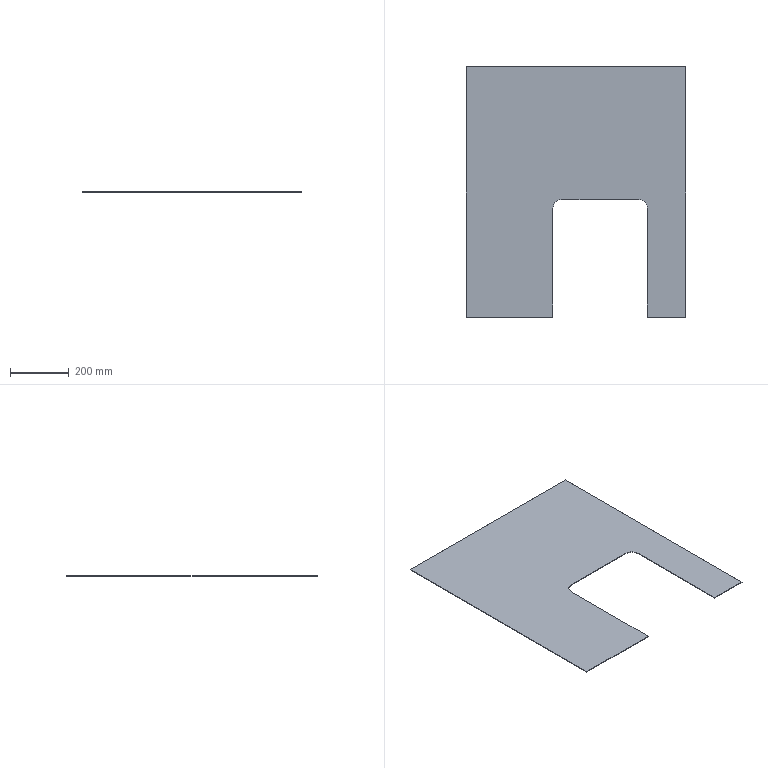Part | STEP file | Part 2 PN_0001_ASM 2 | 1 solid | 12 faces | box 744 x 848.417 x 2 mm | volume 1008010 mm3 | plane 10 | cylinder 2 | commonest cylinder face diameters 60 x2
STEP:
#1=CARTESIAN_POINT('',(23.,847.,0.));
#2=VERTEX_POINT('',#1);
#3=CARTESIAN_POINT('',(23.,-1.417,0.));
#4=VERTEX_POINT('',#3);
#5=CARTESIAN_POINT('',(23.,847.,0.));
#6=DIRECTION('',(0.,-1.,0.));
#7=VECTOR('',#6,1000.);
#8=LINE('',#5,#7);
#9=EDGE_CURVE('',#2,#4,#8,.T.);
#10=ORIENTED_EDGE('',*,*,#9,.F.);
#11=CARTESIAN_POINT('',(23.,847.,-2.));
#12=VERTEX_POINT('',#11);
#13=CARTESIAN_POINT('',(23.,847.,-2.));
#14=DIRECTION('',(0.,0.,1.));
#15=VECTOR('',#14,1000.);
#16=LINE('',#13,#15);
#17=EDGE_CURVE('',#12,#2,#16,.T.);
#18=ORIENTED_EDGE('',*,*,#17,.F.);
#19=CARTESIAN_POINT('',(23.,-1.417,-2.));
#20=VERTEX_POINT('',#19);
#21=CARTESIAN_POINT('',(23.,847.,-2.));
#22=DIRECTION('',(0.,-1.,0.));
#23=VECTOR('',#22,1000.);
#24=LINE('',#21,#23);
#25=EDGE_CURVE('',#12,#20,#24,.T.);
#26=ORIENTED_EDGE('',*,*,#25,.T.);
#27=CARTESIAN_POINT('',(23.,-1.417,-2.));
#28=DIRECTION('',(0.,0.,1.));
#29=VECTOR('',#28,1000.);
#30=LINE('',#27,#29);
#31=EDGE_CURVE('',#20,#4,#30,.T.);
#32=ORIENTED_EDGE('',*,*,#31,.T.);
#33=EDGE_LOOP('',(#10,#18,#26,#32));
#34=FACE_OUTER_BOUND('',#33,.T.);
#35=CARTESIAN_POINT('',(23.,847.,-2.));
#36=DIRECTION('',(-1.,0.,0.));
#37=DIRECTION('',(0.,0.,1.));
#38=AXIS2_PLACEMENT_3D('',#35,#36,#37);
#39=PLANE('',#38);
#40=ADVANCED_FACE('',(#34),#39,.T.);
#41=CARTESIAN_POINT('',(767.,847.,0.));
#42=VERTEX_POINT('',#41);
#43=CARTESIAN_POINT('',(23.,847.,0.));
#44=DIRECTION('',(-1.,0.,0.));
#45=VECTOR('',#44,1000.);
#46=LINE('',#43,#45);
#47=EDGE_CURVE('',#42,#2,#46,.T.);
#48=ORIENTED_EDGE('',*,*,#47,.F.);
#49=CARTESIAN_POINT('',(767.,847.,-2.));
#50=VERTEX_POINT('',#49);
#51=CARTESIAN_POINT('',(767.,847.,-2.));
#52=DIRECTION('',(0.,0.,1.));
#53=VECTOR('',#52,1000.);
#54=LINE('',#51,#53);
#55=EDGE_CURVE('',#50,#42,#54,.T.);
#56=ORIENTED_EDGE('',*,*,#55,.F.);
#57=CARTESIAN_POINT('',(23.,847.,-2.));
#58=DIRECTION('',(-1.,0.,0.));
#59=VECTOR('',#58,1000.);
#60=LINE('',#57,#59);
#61=EDGE_CURVE('',#50,#12,#60,.T.);
#62=ORIENTED_EDGE('',*,*,#61,.T.);
#63=ORIENTED_EDGE('',*,*,#17,.T.);
#64=EDGE_LOOP('',(#48,#56,#62,#63));
#65=FACE_OUTER_BOUND('',#64,.T.);
#66=CARTESIAN_POINT('',(23.,847.,-2.));
#67=DIRECTION('',(0.,1.,0.));
#68=DIRECTION('',(0.,0.,1.));
#69=AXIS2_PLACEMENT_3D('',#66,#67,#68);
#70=PLANE('',#69);
#71=ADVANCED_FACE('',(#65),#70,.T.);
#72=CARTESIAN_POINT('',(767.,-1.417,0.));
#73=VERTEX_POINT('',#72);
#74=CARTESIAN_POINT('',(767.,847.,0.));
#75=DIRECTION('',(0.,1.,0.));
#76=VECTOR('',#75,1000.);
#77=LINE('',#74,#76);
#78=EDGE_CURVE('',#73,#42,#77,.T.);
#79=ORIENTED_EDGE('',*,*,#78,.F.);
#80=CARTESIAN_POINT('',(767.,-1.417,-2.));
#81=VERTEX_POINT('',#80);
#82=CARTESIAN_POINT('',(767.,-1.417,-2.));
#83=DIRECTION('',(0.,0.,1.));
#84=VECTOR('',#83,1000.);
#85=LINE('',#82,#84);
#86=EDGE_CURVE('',#81,#73,#85,.T.);
#87=ORIENTED_EDGE('',*,*,#86,.F.);
#88=CARTESIAN_POINT('',(767.,847.,-2.));
#89=DIRECTION('',(0.,1.,0.));
#90=VECTOR('',#89,1000.);
#91=LINE('',#88,#90);
#92=EDGE_CURVE('',#81,#50,#91,.T.);
#93=ORIENTED_EDGE('',*,*,#92,.T.);
#94=ORIENTED_EDGE('',*,*,#55,.T.);
#95=EDGE_LOOP('',(#79,#87,#93,#94));
#96=FACE_OUTER_BOUND('',#95,.T.);
#97=CARTESIAN_POINT('',(767.,847.,-2.));
#98=DIRECTION('',(1.,0.,0.));
#99=DIRECTION('',(0.,0.,-1.));
#100=AXIS2_PLACEMENT_3D('',#97,#98,#99);
#101=PLANE('',#100);
#102=ADVANCED_FACE('',(#96),#101,.T.);
#103=CARTESIAN_POINT('',(637.185,-1.417,0.));
#104=VERTEX_POINT('',#103);
#105=CARTESIAN_POINT('',(637.185,-1.417,0.));
#106=DIRECTION('',(1.,0.,0.));
#107=VECTOR('',#106,1000.);
#108=LINE('',#105,#107);
#109=EDGE_CURVE('',#104,#73,#108,.T.);
#110=ORIENTED_EDGE('',*,*,#109,.F.);
#111=CARTESIAN_POINT('',(637.185,-1.417,-2.));
#112=VERTEX_POINT('',#111);
#113=CARTESIAN_POINT('',(637.185,-1.417,-2.));
#114=DIRECTION('',(0.,0.,1.));
#115=VECTOR('',#114,1000.);
#116=LINE('',#113,#115);
#117=EDGE_CURVE('',#112,#104,#116,.T.);
#118=ORIENTED_EDGE('',*,*,#117,.F.);
#119=CARTESIAN_POINT('',(637.185,-1.417,-2.));
#120=DIRECTION('',(1.,0.,0.));
#121=VECTOR('',#120,1000.);
#122=LINE('',#119,#121);
#123=EDGE_CURVE('',#112,#81,#122,.T.);
#124=ORIENTED_EDGE('',*,*,#123,.T.);
#125=ORIENTED_EDGE('',*,*,#86,.T.);
#126=EDGE_LOOP('',(#110,#118,#124,#125));
#127=FACE_OUTER_BOUND('',#126,.T.);
#128=CARTESIAN_POINT('',(637.185,-1.417,-2.));
#129=DIRECTION('',(0.,-1.,0.));
#130=DIRECTION('',(0.,0.,-1.));
#131=AXIS2_PLACEMENT_3D('',#128,#129,#130);
#132=PLANE('',#131);
#133=ADVANCED_FACE('',(#127),#132,.T.);
#134=CARTESIAN_POINT('',(637.185,367.054,0.));
#135=VERTEX_POINT('',#134);
#136=CARTESIAN_POINT('',(637.185,-1.417,0.));
#137=DIRECTION('',(0.,-1.,0.));
#138=VECTOR('',#137,1000.);
#139=LINE('',#136,#138);
#140=EDGE_CURVE('',#135,#104,#139,.T.);
#141=ORIENTED_EDGE('',*,*,#140,.F.);
#142=CARTESIAN_POINT('',(637.185,367.054,-2.));
#143=VERTEX_POINT('',#142);
#144=CARTESIAN_POINT('',(637.185,367.054,-2.));
#145=DIRECTION('',(0.,0.,1.));
#146=VECTOR('',#145,1000.);
#147=LINE('',#144,#146);
#148=EDGE_CURVE('',#143,#135,#147,.T.);
#149=ORIENTED_EDGE('',*,*,#148,.F.);
#150=CARTESIAN_POINT('',(637.185,-1.417,-2.));
#151=DIRECTION('',(0.,-1.,0.));
#152=VECTOR('',#151,1000.);
#153=LINE('',#150,#152);
#154=EDGE_CURVE('',#143,#112,#153,.T.);
#155=ORIENTED_EDGE('',*,*,#154,.T.);
#156=ORIENTED_EDGE('',*,*,#117,.T.);
#157=EDGE_LOOP('',(#141,#149,#155,#156));
#158=FACE_OUTER_BOUND('',#157,.T.);
#159=CARTESIAN_POINT('',(637.185,-1.417,-2.));
#160=DIRECTION('',(-1.,0.,0.));
#161=DIRECTION('',(0.,0.,1.));
#162=AXIS2_PLACEMENT_3D('',#159,#160,#161);
#163=PLANE('',#162);
#164=ADVANCED_FACE('',(#158),#163,.T.);
#165=CARTESIAN_POINT('',(607.185,397.054,0.));
#166=VERTEX_POINT('',#165);
#167=CARTESIAN_POINT('',(607.185,367.054,0.));
#168=DIRECTION('',(0.,0.,-1.));
#169=DIRECTION('',(1.,0.,0.));
#170=AXIS2_PLACEMENT_3D('',#167,#168,#169);
#171=CIRCLE('',#170,30.);
#172=EDGE_CURVE('',#166,#135,#171,.T.);
#173=ORIENTED_EDGE('',*,*,#172,.F.);
#174=CARTESIAN_POINT('',(607.185,397.054,-2.));
#175=VERTEX_POINT('',#174);
#176=CARTESIAN_POINT('',(607.185,397.054,-2.));
#177=DIRECTION('',(0.,0.,1.));
#178=VECTOR('',#177,1000.);
#179=LINE('',#176,#178);
#180=EDGE_CURVE('',#175,#166,#179,.T.);
#181=ORIENTED_EDGE('',*,*,#180,.F.);
#182=CARTESIAN_POINT('',(607.185,367.054,-2.));
#183=DIRECTION('',(0.,0.,-1.));
#184=DIRECTION('',(1.,0.,0.));
#185=AXIS2_PLACEMENT_3D('',#182,#183,#184);
#186=CIRCLE('',#185,30.);
#187=EDGE_CURVE('',#175,#143,#186,.T.);
#188=ORIENTED_EDGE('',*,*,#187,.T.);
#189=ORIENTED_EDGE('',*,*,#148,.T.);
#190=EDGE_LOOP('',(#173,#181,#188,#189));
#191=FACE_OUTER_BOUND('',#190,.T.);
#192=CARTESIAN_POINT('',(607.185,367.054,-2.));
#193=DIRECTION('',(0.,0.,1.));
#194=DIRECTION('',(1.,0.,0.));
#195=AXIS2_PLACEMENT_3D('',#192,#193,#194);
#196=CYLINDRICAL_SURFACE('',#195,30.);
#197=ADVANCED_FACE('',(#191),#196,.F.);
#198=CARTESIAN_POINT('',(346.953,397.054,0.));
#199=VERTEX_POINT('',#198);
#200=CARTESIAN_POINT('',(346.953,397.054,0.));
#201=DIRECTION('',(1.,0.,0.));
#202=VECTOR('',#201,1000.);
#203=LINE('',#200,#202);
#204=EDGE_CURVE('',#199,#166,#203,.T.);
#205=ORIENTED_EDGE('',*,*,#204,.F.);
#206=CARTESIAN_POINT('',(346.953,397.054,-2.));
#207=VERTEX_POINT('',#206);
#208=CARTESIAN_POINT('',(346.953,397.054,-2.));
#209=DIRECTION('',(0.,0.,1.));
#210=VECTOR('',#209,1000.);
#211=LINE('',#208,#210);
#212=EDGE_CURVE('',#207,#199,#211,.T.);
#213=ORIENTED_EDGE('',*,*,#212,.F.);
#214=CARTESIAN_POINT('',(346.953,397.054,-2.));
#215=DIRECTION('',(1.,0.,0.));
#216=VECTOR('',#215,1000.);
#217=LINE('',#214,#216);
#218=EDGE_CURVE('',#207,#175,#217,.T.);
#219=ORIENTED_EDGE('',*,*,#218,.T.);
#220=ORIENTED_EDGE('',*,*,#180,.T.);
#221=EDGE_LOOP('',(#205,#213,#219,#220));
#222=FACE_OUTER_BOUND('',#221,.T.);
#223=CARTESIAN_POINT('',(346.953,397.054,-2.));
#224=DIRECTION('',(0.,-1.,0.));
#225=DIRECTION('',(0.,0.,-1.));
#226=AXIS2_PLACEMENT_3D('',#223,#224,#225);
#227=PLANE('',#226);
#228=ADVANCED_FACE('',(#222),#227,.T.);
#229=CARTESIAN_POINT('',(316.953,367.054,0.));
#230=VERTEX_POINT('',#229);
#231=CARTESIAN_POINT('',(346.953,367.054,0.));
#232=DIRECTION('',(0.,0.,-1.));
#233=DIRECTION('',(-1.,0.,0.));
#234=AXIS2_PLACEMENT_3D('',#231,#232,#233);
#235=CIRCLE('',#234,30.);
#236=EDGE_CURVE('',#230,#199,#235,.T.);
#237=ORIENTED_EDGE('',*,*,#236,.F.);
#238=CARTESIAN_POINT('',(316.953,367.054,-2.));
#239=VERTEX_POINT('',#238);
#240=CARTESIAN_POINT('',(316.953,367.054,-2.));
#241=DIRECTION('',(0.,0.,1.));
#242=VECTOR('',#241,1000.);
#243=LINE('',#240,#242);
#244=EDGE_CURVE('',#239,#230,#243,.T.);
#245=ORIENTED_EDGE('',*,*,#244,.F.);
#246=CARTESIAN_POINT('',(346.953,367.054,-2.));
#247=DIRECTION('',(0.,0.,-1.));
#248=DIRECTION('',(-1.,0.,0.));
#249=AXIS2_PLACEMENT_3D('',#246,#247,#248);
#250=CIRCLE('',#249,30.);
#251=EDGE_CURVE('',#239,#207,#250,.T.);
#252=ORIENTED_EDGE('',*,*,#251,.T.);
#253=ORIENTED_EDGE('',*,*,#212,.T.);
#254=EDGE_LOOP('',(#237,#245,#252,#253));
#255=FACE_OUTER_BOUND('',#254,.T.);
#256=CARTESIAN_POINT('',(346.953,367.054,-2.));
#257=DIRECTION('',(0.,0.,1.));
#258=DIRECTION('',(1.,0.,0.));
#259=AXIS2_PLACEMENT_3D('',#256,#257,#258);
#260=CYLINDRICAL_SURFACE('',#259,30.);
#261=ADVANCED_FACE('',(#255),#260,.F.);
#262=CARTESIAN_POINT('',(316.953,-1.417,0.));
#263=VERTEX_POINT('',#262);
#264=CARTESIAN_POINT('',(316.953,-1.417,0.));
#265=DIRECTION('',(0.,1.,0.));
#266=VECTOR('',#265,1000.);
#267=LINE('',#264,#266);
#268=EDGE_CURVE('',#263,#230,#267,.T.);
#269=ORIENTED_EDGE('',*,*,#268,.F.);
#270=CARTESIAN_POINT('',(316.953,-1.417,-2.));
#271=VERTEX_POINT('',#270);
#272=CARTESIAN_POINT('',(316.953,-1.417,-2.));
#273=DIRECTION('',(0.,0.,1.));
#274=VECTOR('',#273,1000.);
#275=LINE('',#272,#274);
#276=EDGE_CURVE('',#271,#263,#275,.T.);
#277=ORIENTED_EDGE('',*,*,#276,.F.);
#278=CARTESIAN_POINT('',(316.953,-1.417,-2.));
#279=DIRECTION('',(0.,1.,0.));
#280=VECTOR('',#279,1000.);
#281=LINE('',#278,#280);
#282=EDGE_CURVE('',#271,#239,#281,.T.);
#283=ORIENTED_EDGE('',*,*,#282,.T.);
#284=ORIENTED_EDGE('',*,*,#244,.T.);
#285=EDGE_LOOP('',(#269,#277,#283,#284));
#286=FACE_OUTER_BOUND('',#285,.T.);
#287=CARTESIAN_POINT('',(316.953,-1.417,-2.));
#288=DIRECTION('',(1.,0.,0.));
#289=DIRECTION('',(0.,0.,-1.));
#290=AXIS2_PLACEMENT_3D('',#287,#288,#289);
#291=PLANE('',#290);
#292=ADVANCED_FACE('',(#286),#291,.T.);
#293=CARTESIAN_POINT('',(23.,-1.417,0.));
#294=DIRECTION('',(1.,0.,0.));
#295=VECTOR('',#294,1000.);
#296=LINE('',#293,#295);
#297=EDGE_CURVE('',#4,#263,#296,.T.);
#298=ORIENTED_EDGE('',*,*,#297,.F.);
#299=ORIENTED_EDGE('',*,*,#31,.F.);
#300=CARTESIAN_POINT('',(23.,-1.417,-2.));
#301=DIRECTION('',(1.,0.,0.));
#302=VECTOR('',#301,1000.);
#303=LINE('',#300,#302);
#304=EDGE_CURVE('',#20,#271,#303,.T.);
#305=ORIENTED_EDGE('',*,*,#304,.T.);
#306=ORIENTED_EDGE('',*,*,#276,.T.);
#307=EDGE_LOOP('',(#298,#299,#305,#306));
#308=FACE_OUTER_BOUND('',#307,.T.);
#309=CARTESIAN_POINT('',(23.,-1.417,-2.));
#310=DIRECTION('',(0.,-1.,0.));
#311=DIRECTION('',(0.,0.,-1.));
#312=AXIS2_PLACEMENT_3D('',#309,#310,#311);
#313=PLANE('',#312);
#314=ADVANCED_FACE('',(#308),#313,.T.);
#315=ORIENTED_EDGE('',*,*,#25,.F.);
#316=ORIENTED_EDGE('',*,*,#61,.F.);
#317=ORIENTED_EDGE('',*,*,#92,.F.);
#318=ORIENTED_EDGE('',*,*,#123,.F.);
#319=ORIENTED_EDGE('',*,*,#154,.F.);
#320=ORIENTED_EDGE('',*,*,#187,.F.);
#321=ORIENTED_EDGE('',*,*,#218,.F.);
#322=ORIENTED_EDGE('',*,*,#251,.F.);
#323=ORIENTED_EDGE('',*,*,#282,.F.);
#324=ORIENTED_EDGE('',*,*,#304,.F.);
#325=EDGE_LOOP('',(#315,#316,#317,#318,#319,#320,#321,#322,#323,#324));
#326=FACE_OUTER_BOUND('',#325,.T.);
#327=CARTESIAN_POINT('',(346.953,367.054,-2.));
#328=DIRECTION('',(0.,0.,-1.));
#329=DIRECTION('',(-1.,0.,0.));
#330=AXIS2_PLACEMENT_3D('',#327,#328,#329);
#331=PLANE('',#330);
#332=ADVANCED_FACE('',(#326),#331,.T.);
#333=ORIENTED_EDGE('',*,*,#9,.T.);
#334=ORIENTED_EDGE('',*,*,#297,.T.);
#335=ORIENTED_EDGE('',*,*,#268,.T.);
#336=ORIENTED_EDGE('',*,*,#236,.T.);
#337=ORIENTED_EDGE('',*,*,#204,.T.);
#338=ORIENTED_EDGE('',*,*,#172,.T.);
#339=ORIENTED_EDGE('',*,*,#140,.T.);
#340=ORIENTED_EDGE('',*,*,#109,.T.);
#341=ORIENTED_EDGE('',*,*,#78,.T.);
#342=ORIENTED_EDGE('',*,*,#47,.T.);
#343=EDGE_LOOP('',(#333,#334,#335,#336,#337,#338,#339,#340,#341,#342));
#344=FACE_OUTER_BOUND('',#343,.T.);
#345=CARTESIAN_POINT('',(346.953,367.054,0.));
#346=DIRECTION('',(0.,0.,-1.));
#347=DIRECTION('',(-1.,0.,0.));
#348=AXIS2_PLACEMENT_3D('',#345,#346,#347);
#349=PLANE('',#348);
#350=ADVANCED_FACE('',(#344),#349,.F.);
#351=CLOSED_SHELL('',(#40,#71,#102,#133,#164,#197,#228,#261,#292,#314,#332,#350));
#352=MANIFOLD_SOLID_BREP('',#351);
#353=CARTESIAN_POINT('',(0.,0.,0.));
#354=DIRECTION('',(0.,0.,1.));
#355=DIRECTION('',(1.,0.,0.));
#356=AXIS2_PLACEMENT_3D('',#353,#354,#355);
#357=(LENGTH_UNIT()NAMED_UNIT(*)SI_UNIT(.MILLI.,.METRE.));
#358=UNCERTAINTY_MEASURE_WITH_UNIT(LENGTH_MEASURE(0.00001),#357,'','');
#359=(NAMED_UNIT(*)PLANE_ANGLE_UNIT()SI_UNIT($,.RADIAN.));
#360=(NAMED_UNIT(*)SI_UNIT($,.STERADIAN.)SOLID_ANGLE_UNIT());
#361=(GEOMETRIC_REPRESENTATION_CONTEXT(3)GLOBAL_UNCERTAINTY_ASSIGNED_CONTEXT((#358))GLOBAL_UNIT_ASSIGNED_CONTEXT((#357,#359,#360))REPRESENTATION_CONTEXT('',''));
#362=ADVANCED_BREP_SHAPE_REPRESENTATION('',(#352,#356),#361);